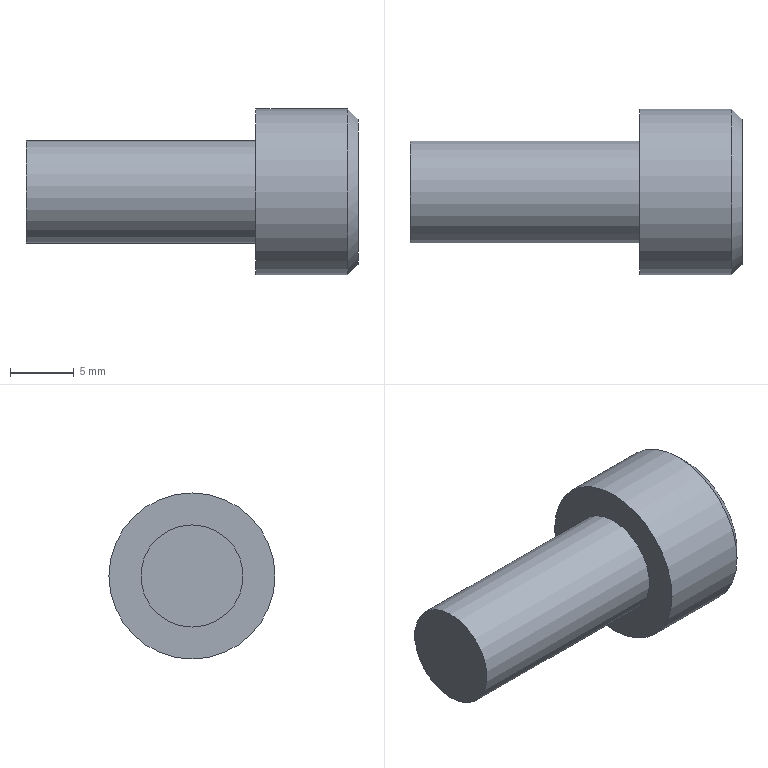Part | NX | features 5003_303_CB8-18 2 | 1 solid | 19 faces | box 26 x 13 x 13 mm | volume 1812 mm3 | plane 15 | cylinder 2 | cone 2 | commonest cylinder face diameters 8 x1 13 x1
STEP:
#1=CARTESIAN_POINT('',(232.525,33.,-57.7));
#2=VERTEX_POINT('',#1);
#3=CARTESIAN_POINT('',(232.525,33.,-52.));
#4=DIRECTION('',(-1.,0.,0.));
#5=DIRECTION('',(0.,0.,-1.));
#6=AXIS2_PLACEMENT_3D('',#3,#4,#5);
#7=CIRCLE('',#6,5.7);
#8=EDGE_CURVE('',#2,#2,#7,.F.);
#9=ORIENTED_EDGE('',*,*,#8,.T.);
#10=EDGE_LOOP('',(#9));
#11=FACE_BOUND('',#10,.T.);
#12=CARTESIAN_POINT('',(232.525,36.464,-52.));
#13=VERTEX_POINT('',#12);
#14=CARTESIAN_POINT('',(232.525,34.732,-49.));
#15=VERTEX_POINT('',#14);
#16=CARTESIAN_POINT('',(232.525,36.464,-52.));
#17=DIRECTION('',(0.,-0.5,0.866));
#18=VECTOR('',#17,1000.);
#19=LINE('',#16,#18);
#20=EDGE_CURVE('',#13,#15,#19,.T.);
#21=ORIENTED_EDGE('',*,*,#20,.F.);
#22=CARTESIAN_POINT('',(232.525,34.732,-55.));
#23=VERTEX_POINT('',#22);
#24=CARTESIAN_POINT('',(232.525,34.732,-55.));
#25=DIRECTION('',(0.,0.5,0.866));
#26=VECTOR('',#25,1000.);
#27=LINE('',#24,#26);
#28=EDGE_CURVE('',#23,#13,#27,.T.);
#29=ORIENTED_EDGE('',*,*,#28,.F.);
#30=CARTESIAN_POINT('',(232.525,31.268,-55.));
#31=VERTEX_POINT('',#30);
#32=CARTESIAN_POINT('',(232.525,31.268,-55.));
#33=DIRECTION('',(0.,1.,0.));
#34=VECTOR('',#33,1000.);
#35=LINE('',#32,#34);
#36=EDGE_CURVE('',#31,#23,#35,.T.);
#37=ORIENTED_EDGE('',*,*,#36,.F.);
#38=CARTESIAN_POINT('',(232.525,29.536,-52.));
#39=VERTEX_POINT('',#38);
#40=CARTESIAN_POINT('',(232.525,29.536,-52.));
#41=DIRECTION('',(0.,0.5,-0.866));
#42=VECTOR('',#41,1000.);
#43=LINE('',#40,#42);
#44=EDGE_CURVE('',#39,#31,#43,.T.);
#45=ORIENTED_EDGE('',*,*,#44,.F.);
#46=CARTESIAN_POINT('',(232.525,31.268,-49.));
#47=VERTEX_POINT('',#46);
#48=CARTESIAN_POINT('',(232.525,31.268,-49.));
#49=DIRECTION('',(0.,-0.5,-0.866));
#50=VECTOR('',#49,1000.);
#51=LINE('',#48,#50);
#52=EDGE_CURVE('',#47,#39,#51,.T.);
#53=ORIENTED_EDGE('',*,*,#52,.F.);
#54=CARTESIAN_POINT('',(232.525,34.732,-49.));
#55=DIRECTION('',(0.,-1.,0.));
#56=VECTOR('',#55,1000.);
#57=LINE('',#54,#56);
#58=EDGE_CURVE('',#15,#47,#57,.T.);
#59=ORIENTED_EDGE('',*,*,#58,.F.);
#60=EDGE_LOOP('',(#21,#29,#37,#45,#53,#59));
#61=FACE_BOUND('',#60,.T.);
#62=CARTESIAN_POINT('',(232.525,26.5,-52.));
#63=DIRECTION('',(-1.,0.,0.));
#64=DIRECTION('',(0.,0.,-1.));
#65=AXIS2_PLACEMENT_3D('',#62,#63,#64);
#66=PLANE('',#65);
#67=ADVANCED_FACE('',(#11,#61),#66,.F.);
#68=CARTESIAN_POINT('',(206.525,33.,-48.));
#69=VERTEX_POINT('',#68);
#70=CARTESIAN_POINT('',(206.525,33.,-52.));
#71=DIRECTION('',(1.,0.,0.));
#72=DIRECTION('',(0.,0.,1.));
#73=AXIS2_PLACEMENT_3D('',#70,#71,#72);
#74=CIRCLE('',#73,4.);
#75=EDGE_CURVE('',#69,#69,#74,.T.);
#76=ORIENTED_EDGE('',*,*,#75,.F.);
#77=EDGE_LOOP('',(#76));
#78=FACE_BOUND('',#77,.T.);
#79=CARTESIAN_POINT('',(206.525,33.,-52.));
#80=DIRECTION('',(1.,0.,0.));
#81=DIRECTION('',(0.,0.,1.));
#82=AXIS2_PLACEMENT_3D('',#79,#80,#81);
#83=PLANE('',#82);
#84=ADVANCED_FACE('',(#78),#83,.F.);
#85=CARTESIAN_POINT('',(224.525,33.,-48.));
#86=VERTEX_POINT('',#85);
#87=CARTESIAN_POINT('',(224.525,33.,-52.));
#88=DIRECTION('',(1.,0.,0.));
#89=DIRECTION('',(0.,0.,1.));
#90=AXIS2_PLACEMENT_3D('',#87,#88,#89);
#91=CIRCLE('',#90,4.);
#92=EDGE_CURVE('',#86,#86,#91,.T.);
#93=ORIENTED_EDGE('',*,*,#92,.F.);
#94=EDGE_LOOP('',(#93));
#95=FACE_BOUND('',#94,.T.);
#96=ORIENTED_EDGE('',*,*,#75,.T.);
#97=EDGE_LOOP('',(#96));
#98=FACE_BOUND('',#97,.T.);
#99=CARTESIAN_POINT('',(232.525,33.,-52.));
#100=DIRECTION('',(1.,0.,0.));
#101=DIRECTION('',(0.,0.,1.));
#102=AXIS2_PLACEMENT_3D('',#99,#100,#101);
#103=CYLINDRICAL_SURFACE('',#102,4.);
#104=ADVANCED_FACE('',(#95,#98),#103,.T.);
#105=CARTESIAN_POINT('',(224.525,33.,-45.5));
#106=VERTEX_POINT('',#105);
#107=CARTESIAN_POINT('',(224.525,33.,-52.));
#108=DIRECTION('',(1.,0.,0.));
#109=DIRECTION('',(0.,0.,1.));
#110=AXIS2_PLACEMENT_3D('',#107,#108,#109);
#111=CIRCLE('',#110,6.5);
#112=EDGE_CURVE('',#106,#106,#111,.T.);
#113=ORIENTED_EDGE('',*,*,#112,.F.);
#114=EDGE_LOOP('',(#113));
#115=FACE_BOUND('',#114,.T.);
#116=ORIENTED_EDGE('',*,*,#92,.T.);
#117=EDGE_LOOP('',(#116));
#118=FACE_BOUND('',#117,.T.);
#119=CARTESIAN_POINT('',(224.525,29.,-52.));
#120=DIRECTION('',(1.,0.,0.));
#121=DIRECTION('',(0.,0.,1.));
#122=AXIS2_PLACEMENT_3D('',#119,#120,#121);
#123=PLANE('',#122);
#124=ADVANCED_FACE('',(#115,#118),#123,.F.);
#125=CARTESIAN_POINT('',(231.725,33.,-58.5));
#126=VERTEX_POINT('',#125);
#127=CARTESIAN_POINT('',(231.725,33.,-52.));
#128=DIRECTION('',(-1.,0.,0.));
#129=DIRECTION('',(0.,0.,-1.));
#130=AXIS2_PLACEMENT_3D('',#127,#128,#129);
#131=CIRCLE('',#130,6.5);
#132=EDGE_CURVE('',#126,#126,#131,.T.);
#133=ORIENTED_EDGE('',*,*,#132,.T.);
#134=EDGE_LOOP('',(#133));
#135=FACE_BOUND('',#134,.T.);
#136=ORIENTED_EDGE('',*,*,#112,.T.);
#137=EDGE_LOOP('',(#136));
#138=FACE_BOUND('',#137,.T.);
#139=CARTESIAN_POINT('',(232.525,33.,-52.));
#140=DIRECTION('',(1.,0.,0.));
#141=DIRECTION('',(0.,0.,1.));
#142=AXIS2_PLACEMENT_3D('',#139,#140,#141);
#143=CYLINDRICAL_SURFACE('',#142,6.5);
#144=ADVANCED_FACE('',(#135,#138),#143,.T.);
#145=ORIENTED_EDGE('',*,*,#132,.F.);
#146=EDGE_LOOP('',(#145));
#147=FACE_BOUND('',#146,.T.);
#148=ORIENTED_EDGE('',*,*,#8,.F.);
#149=EDGE_LOOP('',(#148));
#150=FACE_BOUND('',#149,.T.);
#151=CARTESIAN_POINT('',(232.525,33.,-52.));
#152=DIRECTION('',(-1.,0.,0.));
#153=DIRECTION('',(0.,0.,-1.));
#154=AXIS2_PLACEMENT_3D('',#151,#152,#153);
#155=CONICAL_SURFACE('',#154,5.7,0.7854);
#156=ADVANCED_FACE('',(#147,#150),#155,.T.);
#157=CARTESIAN_POINT('',(228.525,34.732,-55.));
#158=VERTEX_POINT('',#157);
#159=CARTESIAN_POINT('',(228.525,35.598,-53.5));
#160=VERTEX_POINT('',#159);
#161=CARTESIAN_POINT('',(228.525,34.732,-55.));
#162=DIRECTION('',(0.,0.5,0.866));
#163=VECTOR('',#162,1000.);
#164=LINE('',#161,#163);
#165=EDGE_CURVE('',#158,#160,#164,.T.);
#166=ORIENTED_EDGE('',*,*,#165,.F.);
#167=CARTESIAN_POINT('',(228.525,34.732,-55.));
#168=DIRECTION('',(1.,0.,0.));
#169=VECTOR('',#168,1000.);
#170=LINE('',#167,#169);
#171=EDGE_CURVE('',#158,#23,#170,.T.);
#172=ORIENTED_EDGE('',*,*,#171,.T.);
#173=ORIENTED_EDGE('',*,*,#28,.T.);
#174=CARTESIAN_POINT('',(228.525,36.464,-52.));
#175=VERTEX_POINT('',#174);
#176=CARTESIAN_POINT('',(228.525,36.464,-52.));
#177=DIRECTION('',(1.,0.,0.));
#178=VECTOR('',#177,1000.);
#179=LINE('',#176,#178);
#180=EDGE_CURVE('',#175,#13,#179,.T.);
#181=ORIENTED_EDGE('',*,*,#180,.F.);
#182=CARTESIAN_POINT('',(228.525,34.732,-55.));
#183=DIRECTION('',(0.,0.5,0.866));
#184=VECTOR('',#183,1000.);
#185=LINE('',#182,#184);
#186=EDGE_CURVE('',#160,#175,#185,.T.);
#187=ORIENTED_EDGE('',*,*,#186,.F.);
#188=EDGE_LOOP('',(#166,#172,#173,#181,#187));
#189=FACE_BOUND('',#188,.T.);
#190=CARTESIAN_POINT('',(228.525,34.732,-55.));
#191=DIRECTION('',(0.,0.866,-0.5));
#192=DIRECTION('',(0.,-0.5,-0.866));
#193=AXIS2_PLACEMENT_3D('',#190,#191,#192);
#194=PLANE('',#193);
#195=ADVANCED_FACE('',(#189),#194,.F.);
#196=CARTESIAN_POINT('',(228.525,31.268,-55.));
#197=VERTEX_POINT('',#196);
#198=CARTESIAN_POINT('',(228.525,33.,-55.));
#199=VERTEX_POINT('',#198);
#200=CARTESIAN_POINT('',(228.525,31.268,-55.));
#201=DIRECTION('',(0.,1.,0.));
#202=VECTOR('',#201,1000.);
#203=LINE('',#200,#202);
#204=EDGE_CURVE('',#197,#199,#203,.T.);
#205=ORIENTED_EDGE('',*,*,#204,.F.);
#206=CARTESIAN_POINT('',(228.525,31.268,-55.));
#207=DIRECTION('',(1.,0.,0.));
#208=VECTOR('',#207,1000.);
#209=LINE('',#206,#208);
#210=EDGE_CURVE('',#197,#31,#209,.T.);
#211=ORIENTED_EDGE('',*,*,#210,.T.);
#212=ORIENTED_EDGE('',*,*,#36,.T.);
#213=ORIENTED_EDGE('',*,*,#171,.F.);
#214=CARTESIAN_POINT('',(228.525,31.268,-55.));
#215=DIRECTION('',(0.,1.,0.));
#216=VECTOR('',#215,1000.);
#217=LINE('',#214,#216);
#218=EDGE_CURVE('',#199,#158,#217,.T.);
#219=ORIENTED_EDGE('',*,*,#218,.F.);
#220=EDGE_LOOP('',(#205,#211,#212,#213,#219));
#221=FACE_BOUND('',#220,.T.);
#222=CARTESIAN_POINT('',(228.525,31.268,-55.));
#223=DIRECTION('',(0.,0.,-1.));
#224=DIRECTION('',(1.,0.,0.));
#225=AXIS2_PLACEMENT_3D('',#222,#223,#224);
#226=PLANE('',#225);
#227=ADVANCED_FACE('',(#221),#226,.F.);
#228=CARTESIAN_POINT('',(228.525,29.536,-52.));
#229=VERTEX_POINT('',#228);
#230=CARTESIAN_POINT('',(228.525,30.402,-53.5));
#231=VERTEX_POINT('',#230);
#232=CARTESIAN_POINT('',(228.525,29.536,-52.));
#233=DIRECTION('',(0.,0.5,-0.866));
#234=VECTOR('',#233,1000.);
#235=LINE('',#232,#234);
#236=EDGE_CURVE('',#229,#231,#235,.T.);
#237=ORIENTED_EDGE('',*,*,#236,.F.);
#238=CARTESIAN_POINT('',(228.525,29.536,-52.));
#239=DIRECTION('',(1.,0.,0.));
#240=VECTOR('',#239,1000.);
#241=LINE('',#238,#240);
#242=EDGE_CURVE('',#229,#39,#241,.T.);
#243=ORIENTED_EDGE('',*,*,#242,.T.);
#244=ORIENTED_EDGE('',*,*,#44,.T.);
#245=ORIENTED_EDGE('',*,*,#210,.F.);
#246=CARTESIAN_POINT('',(228.525,29.536,-52.));
#247=DIRECTION('',(0.,0.5,-0.866));
#248=VECTOR('',#247,1000.);
#249=LINE('',#246,#248);
#250=EDGE_CURVE('',#231,#197,#249,.T.);
#251=ORIENTED_EDGE('',*,*,#250,.F.);
#252=EDGE_LOOP('',(#237,#243,#244,#245,#251));
#253=FACE_BOUND('',#252,.T.);
#254=CARTESIAN_POINT('',(228.525,29.536,-52.));
#255=DIRECTION('',(0.,-0.866,-0.5));
#256=DIRECTION('',(0.,-0.5,0.866));
#257=AXIS2_PLACEMENT_3D('',#254,#255,#256);
#258=PLANE('',#257);
#259=ADVANCED_FACE('',(#253),#258,.F.);
#260=CARTESIAN_POINT('',(228.525,31.268,-49.));
#261=VERTEX_POINT('',#260);
#262=CARTESIAN_POINT('',(228.525,30.402,-50.5));
#263=VERTEX_POINT('',#262);
#264=CARTESIAN_POINT('',(228.525,31.268,-49.));
#265=DIRECTION('',(0.,-0.5,-0.866));
#266=VECTOR('',#265,1000.);
#267=LINE('',#264,#266);
#268=EDGE_CURVE('',#261,#263,#267,.T.);
#269=ORIENTED_EDGE('',*,*,#268,.F.);
#270=CARTESIAN_POINT('',(228.525,31.268,-49.));
#271=DIRECTION('',(1.,0.,0.));
#272=VECTOR('',#271,1000.);
#273=LINE('',#270,#272);
#274=EDGE_CURVE('',#261,#47,#273,.T.);
#275=ORIENTED_EDGE('',*,*,#274,.T.);
#276=ORIENTED_EDGE('',*,*,#52,.T.);
#277=ORIENTED_EDGE('',*,*,#242,.F.);
#278=CARTESIAN_POINT('',(228.525,31.268,-49.));
#279=DIRECTION('',(0.,-0.5,-0.866));
#280=VECTOR('',#279,1000.);
#281=LINE('',#278,#280);
#282=EDGE_CURVE('',#263,#229,#281,.T.);
#283=ORIENTED_EDGE('',*,*,#282,.F.);
#284=EDGE_LOOP('',(#269,#275,#276,#277,#283));
#285=FACE_BOUND('',#284,.T.);
#286=CARTESIAN_POINT('',(228.525,31.268,-49.));
#287=DIRECTION('',(0.,-0.866,0.5));
#288=DIRECTION('',(0.,0.5,0.866));
#289=AXIS2_PLACEMENT_3D('',#286,#287,#288);
#290=PLANE('',#289);
#291=ADVANCED_FACE('',(#285),#290,.F.);
#292=CARTESIAN_POINT('',(228.525,34.732,-49.));
#293=VERTEX_POINT('',#292);
#294=CARTESIAN_POINT('',(228.525,33.,-49.));
#295=VERTEX_POINT('',#294);
#296=CARTESIAN_POINT('',(228.525,34.732,-49.));
#297=DIRECTION('',(0.,-1.,0.));
#298=VECTOR('',#297,1000.);
#299=LINE('',#296,#298);
#300=EDGE_CURVE('',#293,#295,#299,.T.);
#301=ORIENTED_EDGE('',*,*,#300,.F.);
#302=CARTESIAN_POINT('',(228.525,34.732,-49.));
#303=DIRECTION('',(1.,0.,0.));
#304=VECTOR('',#303,1000.);
#305=LINE('',#302,#304);
#306=EDGE_CURVE('',#293,#15,#305,.T.);
#307=ORIENTED_EDGE('',*,*,#306,.T.);
#308=ORIENTED_EDGE('',*,*,#58,.T.);
#309=ORIENTED_EDGE('',*,*,#274,.F.);
#310=CARTESIAN_POINT('',(228.525,34.732,-49.));
#311=DIRECTION('',(0.,-1.,0.));
#312=VECTOR('',#311,1000.);
#313=LINE('',#310,#312);
#314=EDGE_CURVE('',#295,#261,#313,.T.);
#315=ORIENTED_EDGE('',*,*,#314,.F.);
#316=EDGE_LOOP('',(#301,#307,#308,#309,#315));
#317=FACE_BOUND('',#316,.T.);
#318=CARTESIAN_POINT('',(228.525,34.732,-49.));
#319=DIRECTION('',(0.,0.,1.));
#320=DIRECTION('',(0.,1.,0.));
#321=AXIS2_PLACEMENT_3D('',#318,#319,#320);
#322=PLANE('',#321);
#323=ADVANCED_FACE('',(#317),#322,.F.);
#324=CARTESIAN_POINT('',(228.525,35.598,-50.5));
#325=VERTEX_POINT('',#324);
#326=CARTESIAN_POINT('',(228.525,36.464,-52.));
#327=DIRECTION('',(0.,-0.5,0.866));
#328=VECTOR('',#327,1000.);
#329=LINE('',#326,#328);
#330=EDGE_CURVE('',#175,#325,#329,.T.);
#331=ORIENTED_EDGE('',*,*,#330,.F.);
#332=ORIENTED_EDGE('',*,*,#180,.T.);
#333=ORIENTED_EDGE('',*,*,#20,.T.);
#334=ORIENTED_EDGE('',*,*,#306,.F.);
#335=CARTESIAN_POINT('',(228.525,36.464,-52.));
#336=DIRECTION('',(0.,-0.5,0.866));
#337=VECTOR('',#336,1000.);
#338=LINE('',#335,#337);
#339=EDGE_CURVE('',#325,#293,#338,.T.);
#340=ORIENTED_EDGE('',*,*,#339,.F.);
#341=EDGE_LOOP('',(#331,#332,#333,#334,#340));
#342=FACE_BOUND('',#341,.T.);
#343=CARTESIAN_POINT('',(228.525,36.464,-52.));
#344=DIRECTION('',(0.,0.866,0.5));
#345=DIRECTION('',(0.,0.5,-0.866));
#346=AXIS2_PLACEMENT_3D('',#343,#344,#345);
#347=PLANE('',#346);
#348=ADVANCED_FACE('',(#342),#347,.F.);
#349=ORIENTED_EDGE('',*,*,#314,.T.);
#350=ORIENTED_EDGE('',*,*,#268,.T.);
#351=CARTESIAN_POINT('',(228.525,33.,-52.));
#352=DIRECTION('',(1.,0.,0.));
#353=DIRECTION('',(0.,1.,0.));
#354=AXIS2_PLACEMENT_3D('',#351,#352,#353);
#355=CIRCLE('',#354,3.);
#356=EDGE_CURVE('',#295,#263,#355,.T.);
#357=ORIENTED_EDGE('',*,*,#356,.F.);
#358=EDGE_LOOP('',(#349,#350,#357));
#359=FACE_BOUND('',#358,.T.);
#360=CARTESIAN_POINT('',(228.525,33.,-52.));
#361=DIRECTION('',(1.,0.,0.));
#362=DIRECTION('',(0.,0.,1.));
#363=AXIS2_PLACEMENT_3D('',#360,#361,#362);
#364=PLANE('',#363);
#365=ADVANCED_FACE('',(#359),#364,.T.);
#366=ORIENTED_EDGE('',*,*,#282,.T.);
#367=ORIENTED_EDGE('',*,*,#236,.T.);
#368=CARTESIAN_POINT('',(228.525,33.,-52.));
#369=DIRECTION('',(1.,0.,0.));
#370=DIRECTION('',(0.,1.,0.));
#371=AXIS2_PLACEMENT_3D('',#368,#369,#370);
#372=CIRCLE('',#371,3.);
#373=EDGE_CURVE('',#263,#231,#372,.T.);
#374=ORIENTED_EDGE('',*,*,#373,.F.);
#375=EDGE_LOOP('',(#366,#367,#374));
#376=FACE_BOUND('',#375,.T.);
#377=CARTESIAN_POINT('',(228.525,33.,-52.));
#378=DIRECTION('',(1.,0.,0.));
#379=DIRECTION('',(0.,0.,1.));
#380=AXIS2_PLACEMENT_3D('',#377,#378,#379);
#381=PLANE('',#380);
#382=ADVANCED_FACE('',(#376),#381,.T.);
#383=ORIENTED_EDGE('',*,*,#250,.T.);
#384=ORIENTED_EDGE('',*,*,#204,.T.);
#385=CARTESIAN_POINT('',(228.525,33.,-52.));
#386=DIRECTION('',(1.,0.,0.));
#387=DIRECTION('',(0.,1.,0.));
#388=AXIS2_PLACEMENT_3D('',#385,#386,#387);
#389=CIRCLE('',#388,3.);
#390=EDGE_CURVE('',#231,#199,#389,.T.);
#391=ORIENTED_EDGE('',*,*,#390,.F.);
#392=EDGE_LOOP('',(#383,#384,#391));
#393=FACE_BOUND('',#392,.T.);
#394=CARTESIAN_POINT('',(228.525,33.,-52.));
#395=DIRECTION('',(1.,0.,0.));
#396=DIRECTION('',(0.,0.,1.));
#397=AXIS2_PLACEMENT_3D('',#394,#395,#396);
#398=PLANE('',#397);
#399=ADVANCED_FACE('',(#393),#398,.T.);
#400=ORIENTED_EDGE('',*,*,#218,.T.);
#401=ORIENTED_EDGE('',*,*,#165,.T.);
#402=CARTESIAN_POINT('',(228.525,33.,-52.));
#403=DIRECTION('',(1.,0.,0.));
#404=DIRECTION('',(0.,1.,0.));
#405=AXIS2_PLACEMENT_3D('',#402,#403,#404);
#406=CIRCLE('',#405,3.);
#407=EDGE_CURVE('',#199,#160,#406,.T.);
#408=ORIENTED_EDGE('',*,*,#407,.F.);
#409=EDGE_LOOP('',(#400,#401,#408));
#410=FACE_BOUND('',#409,.T.);
#411=CARTESIAN_POINT('',(228.525,33.,-52.));
#412=DIRECTION('',(1.,0.,0.));
#413=DIRECTION('',(0.,0.,1.));
#414=AXIS2_PLACEMENT_3D('',#411,#412,#413);
#415=PLANE('',#414);
#416=ADVANCED_FACE('',(#410),#415,.T.);
#417=ORIENTED_EDGE('',*,*,#186,.T.);
#418=ORIENTED_EDGE('',*,*,#330,.T.);
#419=CARTESIAN_POINT('',(228.525,33.,-52.));
#420=DIRECTION('',(1.,0.,0.));
#421=DIRECTION('',(0.,1.,0.));
#422=AXIS2_PLACEMENT_3D('',#419,#420,#421);
#423=CIRCLE('',#422,3.);
#424=EDGE_CURVE('',#160,#325,#423,.T.);
#425=ORIENTED_EDGE('',*,*,#424,.F.);
#426=EDGE_LOOP('',(#417,#418,#425));
#427=FACE_BOUND('',#426,.T.);
#428=CARTESIAN_POINT('',(228.525,33.,-52.));
#429=DIRECTION('',(1.,0.,0.));
#430=DIRECTION('',(0.,0.,1.));
#431=AXIS2_PLACEMENT_3D('',#428,#429,#430);
#432=PLANE('',#431);
#433=ADVANCED_FACE('',(#427),#432,.T.);
#434=ORIENTED_EDGE('',*,*,#339,.T.);
#435=ORIENTED_EDGE('',*,*,#300,.T.);
#436=CARTESIAN_POINT('',(228.525,33.,-52.));
#437=DIRECTION('',(1.,0.,0.));
#438=DIRECTION('',(0.,1.,0.));
#439=AXIS2_PLACEMENT_3D('',#436,#437,#438);
#440=CIRCLE('',#439,3.);
#441=EDGE_CURVE('',#325,#295,#440,.T.);
#442=ORIENTED_EDGE('',*,*,#441,.F.);
#443=EDGE_LOOP('',(#434,#435,#442));
#444=FACE_BOUND('',#443,.T.);
#445=CARTESIAN_POINT('',(228.525,33.,-52.));
#446=DIRECTION('',(1.,0.,0.));
#447=DIRECTION('',(0.,0.,1.));
#448=AXIS2_PLACEMENT_3D('',#445,#446,#447);
#449=PLANE('',#448);
#450=ADVANCED_FACE('',(#444),#449,.T.);
#451=ORIENTED_EDGE('',*,*,#441,.T.);
#452=ORIENTED_EDGE('',*,*,#356,.T.);
#453=ORIENTED_EDGE('',*,*,#373,.T.);
#454=ORIENTED_EDGE('',*,*,#390,.T.);
#455=ORIENTED_EDGE('',*,*,#407,.T.);
#456=ORIENTED_EDGE('',*,*,#424,.T.);
#457=EDGE_LOOP('',(#451,#452,#453,#454,#455,#456));
#458=FACE_BOUND('',#457,.T.);
#459=CARTESIAN_POINT('',(226.722,33.,-52.));
#460=VERTEX_POINT('',#459);
#461=VERTEX_LOOP('',#460);
#462=FACE_BOUND('',#461,.T.);
#463=CARTESIAN_POINT('',(226.722,33.,-52.));
#464=DIRECTION('',(1.,0.,0.));
#465=DIRECTION('',(0.,1.,0.));
#466=AXIS2_PLACEMENT_3D('',#463,#464,#465);
#467=CONICAL_SURFACE('',#466,0.,1.03);
#468=ADVANCED_FACE('',(#458,#462),#467,.F.);
#469=CLOSED_SHELL('',(#67,#84,#104,#124,#144,#156,#195,#227,#259,#291,#323,#348,#365,#382,#399,#416,#433,#450,#468));
#470=MANIFOLD_SOLID_BREP('',#469);
#471=(LENGTH_UNIT()NAMED_UNIT(*)SI_UNIT(.MILLI.,.METRE.));
#472=UNCERTAINTY_MEASURE_WITH_UNIT(LENGTH_MEASURE(0.00001),#471,'','');
#473=(NAMED_UNIT(*)PLANE_ANGLE_UNIT()SI_UNIT($,.RADIAN.));
#474=(NAMED_UNIT(*)SI_UNIT($,.STERADIAN.)SOLID_ANGLE_UNIT());
#475=(GEOMETRIC_REPRESENTATION_CONTEXT(3)GLOBAL_UNCERTAINTY_ASSIGNED_CONTEXT((#472))GLOBAL_UNIT_ASSIGNED_CONTEXT((#471,#473,#474))REPRESENTATION_CONTEXT('',''));
#476=ADVANCED_BREP_SHAPE_REPRESENTATION('',(#470),#475);